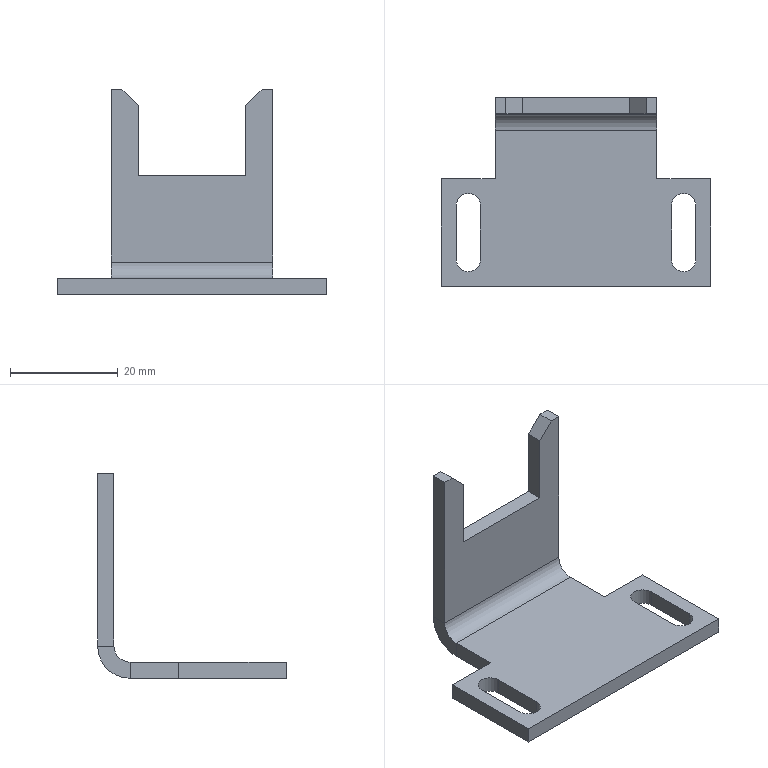Part | NX | features BREP 1 | 1 solid | 32 faces | box 50 x 35 x 38 mm | volume 5974 mm3 | plane 26 | cylinder 6 | commonest cylinder face diameters 4.5 x4 6 x1 12 x1
STEP:
#1=CARTESIAN_POINT('',(-13.,-3.,38.));
#2=VERTEX_POINT('',#1);
#3=CARTESIAN_POINT('',(-15.,-3.,38.));
#4=VERTEX_POINT('',#3);
#5=CARTESIAN_POINT('',(15.,-3.,38.));
#6=DIRECTION('',(-1.,0.,0.));
#7=VECTOR('',#6,1000.);
#8=LINE('',#5,#7);
#9=EDGE_CURVE('',#2,#4,#8,.T.);
#10=ORIENTED_EDGE('',*,*,#9,.F.);
#11=CARTESIAN_POINT('',(-13.,0.,38.));
#12=VERTEX_POINT('',#11);
#13=CARTESIAN_POINT('',(-13.,0.,38.));
#14=DIRECTION('',(0.,1.,0.));
#15=VECTOR('',#14,1000.);
#16=LINE('',#13,#15);
#17=EDGE_CURVE('',#2,#12,#16,.T.);
#18=ORIENTED_EDGE('',*,*,#17,.T.);
#19=CARTESIAN_POINT('',(-15.,0.,38.));
#20=VERTEX_POINT('',#19);
#21=CARTESIAN_POINT('',(15.,0.,38.));
#22=DIRECTION('',(-1.,0.,0.));
#23=VECTOR('',#22,1000.);
#24=LINE('',#21,#23);
#25=EDGE_CURVE('',#12,#20,#24,.T.);
#26=ORIENTED_EDGE('',*,*,#25,.T.);
#27=CARTESIAN_POINT('',(-15.,-3.,38.));
#28=DIRECTION('',(0.,1.,0.));
#29=VECTOR('',#28,1000.);
#30=LINE('',#27,#29);
#31=EDGE_CURVE('',#4,#20,#30,.T.);
#32=ORIENTED_EDGE('',*,*,#31,.F.);
#33=EDGE_LOOP('',(#10,#18,#26,#32));
#34=FACE_BOUND('',#33,.T.);
#35=CARTESIAN_POINT('',(15.,-3.,38.));
#36=DIRECTION('',(0.,0.,1.));
#37=DIRECTION('',(-1.,0.,0.));
#38=AXIS2_PLACEMENT_3D('',#35,#36,#37);
#39=PLANE('',#38);
#40=ADVANCED_FACE('',(#34),#39,.T.);
#41=CARTESIAN_POINT('',(15.,-6.,0.));
#42=VERTEX_POINT('',#41);
#43=CARTESIAN_POINT('',(15.,-6.,3.));
#44=VERTEX_POINT('',#43);
#45=CARTESIAN_POINT('',(15.,-6.,0.));
#46=DIRECTION('',(0.,0.,1.));
#47=VECTOR('',#46,1000.);
#48=LINE('',#45,#47);
#49=EDGE_CURVE('',#42,#44,#48,.T.);
#50=ORIENTED_EDGE('',*,*,#49,.F.);
#51=CARTESIAN_POINT('',(15.,0.,6.));
#52=VERTEX_POINT('',#51);
#53=CARTESIAN_POINT('',(15.,-6.,6.));
#54=DIRECTION('',(-1.,0.,0.));
#55=DIRECTION('',(0.,0.,-1.));
#56=AXIS2_PLACEMENT_3D('',#53,#54,#55);
#57=CIRCLE('',#56,6.);
#58=EDGE_CURVE('',#52,#42,#57,.T.);
#59=ORIENTED_EDGE('',*,*,#58,.F.);
#60=CARTESIAN_POINT('',(15.,-3.,6.));
#61=VERTEX_POINT('',#60);
#62=CARTESIAN_POINT('',(15.,-3.,6.));
#63=DIRECTION('',(0.,1.,0.));
#64=VECTOR('',#63,1000.);
#65=LINE('',#62,#64);
#66=EDGE_CURVE('',#61,#52,#65,.T.);
#67=ORIENTED_EDGE('',*,*,#66,.F.);
#68=CARTESIAN_POINT('',(15.,-6.,6.));
#69=DIRECTION('',(-1.,0.,0.));
#70=DIRECTION('',(0.,0.,-1.));
#71=AXIS2_PLACEMENT_3D('',#68,#69,#70);
#72=CIRCLE('',#71,3.);
#73=EDGE_CURVE('',#61,#44,#72,.T.);
#74=ORIENTED_EDGE('',*,*,#73,.T.);
#75=EDGE_LOOP('',(#50,#59,#67,#74));
#76=FACE_BOUND('',#75,.T.);
#77=CARTESIAN_POINT('',(15.,-6.,0.));
#78=DIRECTION('',(1.,0.,0.));
#79=DIRECTION('',(0.,0.,1.));
#80=AXIS2_PLACEMENT_3D('',#77,#78,#79);
#81=PLANE('',#80);
#82=ADVANCED_FACE('',(#76),#81,.T.);
#83=CARTESIAN_POINT('',(15.,-15.,0.));
#84=VERTEX_POINT('',#83);
#85=CARTESIAN_POINT('',(15.,-15.,3.));
#86=VERTEX_POINT('',#85);
#87=CARTESIAN_POINT('',(15.,-15.,6.));
#88=DIRECTION('',(0.,0.,1.));
#89=VECTOR('',#88,1000.);
#90=LINE('',#87,#89);
#91=EDGE_CURVE('',#84,#86,#90,.T.);
#92=ORIENTED_EDGE('',*,*,#91,.F.);
#93=CARTESIAN_POINT('',(15.,0.,0.));
#94=DIRECTION('',(0.,-1.,0.));
#95=VECTOR('',#94,1000.);
#96=LINE('',#93,#95);
#97=EDGE_CURVE('',#42,#84,#96,.T.);
#98=ORIENTED_EDGE('',*,*,#97,.F.);
#99=ORIENTED_EDGE('',*,*,#49,.T.);
#100=CARTESIAN_POINT('',(15.,0.,3.));
#101=DIRECTION('',(0.,-1.,0.));
#102=VECTOR('',#101,1000.);
#103=LINE('',#100,#102);
#104=EDGE_CURVE('',#44,#86,#103,.T.);
#105=ORIENTED_EDGE('',*,*,#104,.T.);
#106=EDGE_LOOP('',(#92,#98,#99,#105));
#107=FACE_BOUND('',#106,.T.);
#108=CARTESIAN_POINT('',(15.,-3.,6.));
#109=DIRECTION('',(1.,0.,0.));
#110=DIRECTION('',(0.,0.,1.));
#111=AXIS2_PLACEMENT_3D('',#108,#109,#110);
#112=PLANE('',#111);
#113=ADVANCED_FACE('',(#107),#112,.T.);
#114=CARTESIAN_POINT('',(-15.,0.,6.));
#115=VERTEX_POINT('',#114);
#116=CARTESIAN_POINT('',(-15.,-3.,6.));
#117=VERTEX_POINT('',#116);
#118=CARTESIAN_POINT('',(-15.,0.,6.));
#119=DIRECTION('',(0.,-1.,0.));
#120=VECTOR('',#119,1000.);
#121=LINE('',#118,#120);
#122=EDGE_CURVE('',#115,#117,#121,.T.);
#123=ORIENTED_EDGE('',*,*,#122,.F.);
#124=CARTESIAN_POINT('',(-15.,-6.,0.));
#125=VERTEX_POINT('',#124);
#126=CARTESIAN_POINT('',(-15.,-6.,6.));
#127=DIRECTION('',(-1.,0.,0.));
#128=DIRECTION('',(0.,0.,-1.));
#129=AXIS2_PLACEMENT_3D('',#126,#127,#128);
#130=CIRCLE('',#129,6.);
#131=EDGE_CURVE('',#115,#125,#130,.T.);
#132=ORIENTED_EDGE('',*,*,#131,.T.);
#133=CARTESIAN_POINT('',(-15.,-6.,3.));
#134=VERTEX_POINT('',#133);
#135=CARTESIAN_POINT('',(-15.,-6.,3.));
#136=DIRECTION('',(0.,0.,-1.));
#137=VECTOR('',#136,1000.);
#138=LINE('',#135,#137);
#139=EDGE_CURVE('',#134,#125,#138,.T.);
#140=ORIENTED_EDGE('',*,*,#139,.F.);
#141=CARTESIAN_POINT('',(-15.,-6.,6.));
#142=DIRECTION('',(-1.,0.,0.));
#143=DIRECTION('',(0.,0.,-1.));
#144=AXIS2_PLACEMENT_3D('',#141,#142,#143);
#145=CIRCLE('',#144,3.);
#146=EDGE_CURVE('',#117,#134,#145,.T.);
#147=ORIENTED_EDGE('',*,*,#146,.F.);
#148=EDGE_LOOP('',(#123,#132,#140,#147));
#149=FACE_BOUND('',#148,.T.);
#150=CARTESIAN_POINT('',(-15.,0.,6.));
#151=DIRECTION('',(-1.,0.,0.));
#152=DIRECTION('',(0.,0.,-1.));
#153=AXIS2_PLACEMENT_3D('',#150,#151,#152);
#154=PLANE('',#153);
#155=ADVANCED_FACE('',(#149),#154,.T.);
#156=CARTESIAN_POINT('',(-15.,0.,38.));
#157=DIRECTION('',(0.,0.,-1.));
#158=VECTOR('',#157,1000.);
#159=LINE('',#156,#158);
#160=EDGE_CURVE('',#20,#115,#159,.T.);
#161=ORIENTED_EDGE('',*,*,#160,.T.);
#162=ORIENTED_EDGE('',*,*,#122,.T.);
#163=CARTESIAN_POINT('',(-15.,-3.,38.));
#164=DIRECTION('',(0.,0.,-1.));
#165=VECTOR('',#164,1000.);
#166=LINE('',#163,#165);
#167=EDGE_CURVE('',#4,#117,#166,.T.);
#168=ORIENTED_EDGE('',*,*,#167,.F.);
#169=ORIENTED_EDGE('',*,*,#31,.T.);
#170=EDGE_LOOP('',(#161,#162,#168,#169));
#171=FACE_BOUND('',#170,.T.);
#172=CARTESIAN_POINT('',(-15.,-6.,3.));
#173=DIRECTION('',(-1.,0.,0.));
#174=DIRECTION('',(0.,0.,-1.));
#175=AXIS2_PLACEMENT_3D('',#172,#173,#174);
#176=PLANE('',#175);
#177=ADVANCED_FACE('',(#171),#176,.T.);
#178=CARTESIAN_POINT('',(17.75,-30.,3.));
#179=VERTEX_POINT('',#178);
#180=CARTESIAN_POINT('',(22.25,-30.,3.));
#181=VERTEX_POINT('',#180);
#182=CARTESIAN_POINT('',(20.,-30.,3.));
#183=DIRECTION('',(0.,0.,1.));
#184=DIRECTION('',(1.,0.,0.));
#185=AXIS2_PLACEMENT_3D('',#182,#183,#184);
#186=CIRCLE('',#185,2.25);
#187=EDGE_CURVE('',#179,#181,#186,.T.);
#188=ORIENTED_EDGE('',*,*,#187,.F.);
#189=CARTESIAN_POINT('',(17.75,-20.,3.));
#190=VERTEX_POINT('',#189);
#191=CARTESIAN_POINT('',(17.75,-20.,3.));
#192=DIRECTION('',(0.,-1.,0.));
#193=VECTOR('',#192,1000.);
#194=LINE('',#191,#193);
#195=EDGE_CURVE('',#190,#179,#194,.T.);
#196=ORIENTED_EDGE('',*,*,#195,.F.);
#197=CARTESIAN_POINT('',(22.25,-20.,3.));
#198=VERTEX_POINT('',#197);
#199=CARTESIAN_POINT('',(20.,-20.,3.));
#200=DIRECTION('',(0.,0.,1.));
#201=DIRECTION('',(1.,0.,0.));
#202=AXIS2_PLACEMENT_3D('',#199,#200,#201);
#203=CIRCLE('',#202,2.25);
#204=EDGE_CURVE('',#198,#190,#203,.T.);
#205=ORIENTED_EDGE('',*,*,#204,.F.);
#206=CARTESIAN_POINT('',(22.25,-20.,3.));
#207=DIRECTION('',(0.,1.,0.));
#208=VECTOR('',#207,1000.);
#209=LINE('',#206,#208);
#210=EDGE_CURVE('',#181,#198,#209,.T.);
#211=ORIENTED_EDGE('',*,*,#210,.F.);
#212=EDGE_LOOP('',(#188,#196,#205,#211));
#213=FACE_BOUND('',#212,.T.);
#214=CARTESIAN_POINT('',(-22.25,-30.,3.));
#215=VERTEX_POINT('',#214);
#216=CARTESIAN_POINT('',(-17.75,-30.,3.));
#217=VERTEX_POINT('',#216);
#218=CARTESIAN_POINT('',(-20.,-30.,3.));
#219=DIRECTION('',(0.,0.,1.));
#220=DIRECTION('',(1.,0.,0.));
#221=AXIS2_PLACEMENT_3D('',#218,#219,#220);
#222=CIRCLE('',#221,2.25);
#223=EDGE_CURVE('',#215,#217,#222,.T.);
#224=ORIENTED_EDGE('',*,*,#223,.F.);
#225=CARTESIAN_POINT('',(-22.25,-20.,3.));
#226=VERTEX_POINT('',#225);
#227=CARTESIAN_POINT('',(-22.25,-20.,3.));
#228=DIRECTION('',(0.,-1.,0.));
#229=VECTOR('',#228,1000.);
#230=LINE('',#227,#229);
#231=EDGE_CURVE('',#226,#215,#230,.T.);
#232=ORIENTED_EDGE('',*,*,#231,.F.);
#233=CARTESIAN_POINT('',(-17.75,-20.,3.));
#234=VERTEX_POINT('',#233);
#235=CARTESIAN_POINT('',(-20.,-20.,3.));
#236=DIRECTION('',(0.,0.,1.));
#237=DIRECTION('',(1.,0.,0.));
#238=AXIS2_PLACEMENT_3D('',#235,#236,#237);
#239=CIRCLE('',#238,2.25);
#240=EDGE_CURVE('',#234,#226,#239,.T.);
#241=ORIENTED_EDGE('',*,*,#240,.F.);
#242=CARTESIAN_POINT('',(-17.75,-20.,3.));
#243=DIRECTION('',(0.,1.,0.));
#244=VECTOR('',#243,1000.);
#245=LINE('',#242,#244);
#246=EDGE_CURVE('',#217,#234,#245,.T.);
#247=ORIENTED_EDGE('',*,*,#246,.F.);
#248=EDGE_LOOP('',(#224,#232,#241,#247));
#249=FACE_BOUND('',#248,.T.);
#250=CARTESIAN_POINT('',(-15.,-15.,3.));
#251=VERTEX_POINT('',#250);
#252=CARTESIAN_POINT('',(-15.,0.,3.));
#253=DIRECTION('',(0.,-1.,0.));
#254=VECTOR('',#253,1000.);
#255=LINE('',#252,#254);
#256=EDGE_CURVE('',#134,#251,#255,.T.);
#257=ORIENTED_EDGE('',*,*,#256,.T.);
#258=CARTESIAN_POINT('',(-25.,-15.,3.));
#259=VERTEX_POINT('',#258);
#260=CARTESIAN_POINT('',(25.,-15.,3.));
#261=DIRECTION('',(-1.,0.,0.));
#262=VECTOR('',#261,1000.);
#263=LINE('',#260,#262);
#264=EDGE_CURVE('',#251,#259,#263,.T.);
#265=ORIENTED_EDGE('',*,*,#264,.T.);
#266=CARTESIAN_POINT('',(-25.,-35.,3.));
#267=VERTEX_POINT('',#266);
#268=CARTESIAN_POINT('',(-25.,-15.,3.));
#269=DIRECTION('',(0.,-1.,0.));
#270=VECTOR('',#269,1000.);
#271=LINE('',#268,#270);
#272=EDGE_CURVE('',#259,#267,#271,.T.);
#273=ORIENTED_EDGE('',*,*,#272,.T.);
#274=CARTESIAN_POINT('',(25.,-35.,3.));
#275=VERTEX_POINT('',#274);
#276=CARTESIAN_POINT('',(15.,-35.,3.));
#277=DIRECTION('',(-1.,0.,0.));
#278=VECTOR('',#277,1000.);
#279=LINE('',#276,#278);
#280=EDGE_CURVE('',#275,#267,#279,.T.);
#281=ORIENTED_EDGE('',*,*,#280,.F.);
#282=CARTESIAN_POINT('',(25.,-15.,3.));
#283=VERTEX_POINT('',#282);
#284=CARTESIAN_POINT('',(25.,-15.,3.));
#285=DIRECTION('',(0.,1.,0.));
#286=VECTOR('',#285,1000.);
#287=LINE('',#284,#286);
#288=EDGE_CURVE('',#275,#283,#287,.T.);
#289=ORIENTED_EDGE('',*,*,#288,.T.);
#290=CARTESIAN_POINT('',(25.,-15.,3.));
#291=DIRECTION('',(-1.,0.,0.));
#292=VECTOR('',#291,1000.);
#293=LINE('',#290,#292);
#294=EDGE_CURVE('',#283,#86,#293,.T.);
#295=ORIENTED_EDGE('',*,*,#294,.T.);
#296=ORIENTED_EDGE('',*,*,#104,.F.);
#297=CARTESIAN_POINT('',(15.,-6.,3.));
#298=DIRECTION('',(-1.,0.,0.));
#299=VECTOR('',#298,1000.);
#300=LINE('',#297,#299);
#301=EDGE_CURVE('',#44,#134,#300,.T.);
#302=ORIENTED_EDGE('',*,*,#301,.T.);
#303=EDGE_LOOP('',(#257,#265,#273,#281,#289,#295,#296,#302));
#304=FACE_BOUND('',#303,.T.);
#305=CARTESIAN_POINT('',(15.,0.,3.));
#306=DIRECTION('',(0.,0.,-1.));
#307=DIRECTION('',(0.,-1.,0.));
#308=AXIS2_PLACEMENT_3D('',#305,#306,#307);
#309=PLANE('',#308);
#310=ADVANCED_FACE('',(#213,#249,#304),#309,.F.);
#311=ORIENTED_EDGE('',*,*,#280,.T.);
#312=CARTESIAN_POINT('',(-25.,-35.,0.));
#313=VERTEX_POINT('',#312);
#314=CARTESIAN_POINT('',(-25.,-35.,-53.852));
#315=DIRECTION('',(0.,0.,1.));
#316=VECTOR('',#315,1000.);
#317=LINE('',#314,#316);
#318=EDGE_CURVE('',#313,#267,#317,.T.);
#319=ORIENTED_EDGE('',*,*,#318,.F.);
#320=CARTESIAN_POINT('',(25.,-35.,0.));
#321=VERTEX_POINT('',#320);
#322=CARTESIAN_POINT('',(15.,-35.,0.));
#323=DIRECTION('',(-1.,0.,0.));
#324=VECTOR('',#323,1000.);
#325=LINE('',#322,#324);
#326=EDGE_CURVE('',#321,#313,#325,.T.);
#327=ORIENTED_EDGE('',*,*,#326,.F.);
#328=CARTESIAN_POINT('',(25.,-35.,-53.852));
#329=DIRECTION('',(0.,0.,1.));
#330=VECTOR('',#329,1000.);
#331=LINE('',#328,#330);
#332=EDGE_CURVE('',#321,#275,#331,.T.);
#333=ORIENTED_EDGE('',*,*,#332,.T.);
#334=EDGE_LOOP('',(#311,#319,#327,#333));
#335=FACE_BOUND('',#334,.T.);
#336=CARTESIAN_POINT('',(15.,-35.,0.));
#337=DIRECTION('',(0.,-1.,0.));
#338=DIRECTION('',(0.,0.,1.));
#339=AXIS2_PLACEMENT_3D('',#336,#337,#338);
#340=PLANE('',#339);
#341=ADVANCED_FACE('',(#335),#340,.T.);
#342=CARTESIAN_POINT('',(17.75,-20.,0.));
#343=VERTEX_POINT('',#342);
#344=CARTESIAN_POINT('',(17.75,-30.,0.));
#345=VERTEX_POINT('',#344);
#346=CARTESIAN_POINT('',(17.75,-20.,0.));
#347=DIRECTION('',(0.,-1.,0.));
#348=VECTOR('',#347,1000.);
#349=LINE('',#346,#348);
#350=EDGE_CURVE('',#343,#345,#349,.T.);
#351=ORIENTED_EDGE('',*,*,#350,.T.);
#352=CARTESIAN_POINT('',(22.25,-30.,0.));
#353=VERTEX_POINT('',#352);
#354=CARTESIAN_POINT('',(20.,-30.,0.));
#355=DIRECTION('',(0.,0.,1.));
#356=DIRECTION('',(0.,1.,0.));
#357=AXIS2_PLACEMENT_3D('',#354,#355,#356);
#358=CIRCLE('',#357,2.25);
#359=EDGE_CURVE('',#345,#353,#358,.T.);
#360=ORIENTED_EDGE('',*,*,#359,.T.);
#361=CARTESIAN_POINT('',(22.25,-20.,0.));
#362=VERTEX_POINT('',#361);
#363=CARTESIAN_POINT('',(22.25,-20.,0.));
#364=DIRECTION('',(0.,1.,0.));
#365=VECTOR('',#364,1000.);
#366=LINE('',#363,#365);
#367=EDGE_CURVE('',#353,#362,#366,.T.);
#368=ORIENTED_EDGE('',*,*,#367,.T.);
#369=CARTESIAN_POINT('',(20.,-20.,0.));
#370=DIRECTION('',(0.,0.,1.));
#371=DIRECTION('',(0.,1.,0.));
#372=AXIS2_PLACEMENT_3D('',#369,#370,#371);
#373=CIRCLE('',#372,2.25);
#374=EDGE_CURVE('',#362,#343,#373,.T.);
#375=ORIENTED_EDGE('',*,*,#374,.T.);
#376=EDGE_LOOP('',(#351,#360,#368,#375));
#377=FACE_BOUND('',#376,.T.);
#378=CARTESIAN_POINT('',(-22.25,-20.,0.));
#379=VERTEX_POINT('',#378);
#380=CARTESIAN_POINT('',(-22.25,-30.,0.));
#381=VERTEX_POINT('',#380);
#382=CARTESIAN_POINT('',(-22.25,-20.,0.));
#383=DIRECTION('',(0.,-1.,0.));
#384=VECTOR('',#383,1000.);
#385=LINE('',#382,#384);
#386=EDGE_CURVE('',#379,#381,#385,.T.);
#387=ORIENTED_EDGE('',*,*,#386,.T.);
#388=CARTESIAN_POINT('',(-17.75,-30.,0.));
#389=VERTEX_POINT('',#388);
#390=CARTESIAN_POINT('',(-20.,-30.,0.));
#391=DIRECTION('',(0.,0.,1.));
#392=DIRECTION('',(0.,1.,0.));
#393=AXIS2_PLACEMENT_3D('',#390,#391,#392);
#394=CIRCLE('',#393,2.25);
#395=EDGE_CURVE('',#381,#389,#394,.T.);
#396=ORIENTED_EDGE('',*,*,#395,.T.);
#397=CARTESIAN_POINT('',(-17.75,-20.,0.));
#398=VERTEX_POINT('',#397);
#399=CARTESIAN_POINT('',(-17.75,-20.,0.));
#400=DIRECTION('',(0.,1.,0.));
#401=VECTOR('',#400,1000.);
#402=LINE('',#399,#401);
#403=EDGE_CURVE('',#389,#398,#402,.T.);
#404=ORIENTED_EDGE('',*,*,#403,.T.);
#405=CARTESIAN_POINT('',(-20.,-20.,0.));
#406=DIRECTION('',(0.,0.,1.));
#407=DIRECTION('',(0.,1.,0.));
#408=AXIS2_PLACEMENT_3D('',#405,#406,#407);
#409=CIRCLE('',#408,2.25);
#410=EDGE_CURVE('',#398,#379,#409,.T.);
#411=ORIENTED_EDGE('',*,*,#410,.T.);
#412=EDGE_LOOP('',(#387,#396,#404,#411));
#413=FACE_BOUND('',#412,.T.);
#414=ORIENTED_EDGE('',*,*,#97,.T.);
#415=CARTESIAN_POINT('',(25.,-15.,0.));
#416=VERTEX_POINT('',#415);
#417=CARTESIAN_POINT('',(25.,-15.,0.));
#418=DIRECTION('',(-1.,0.,0.));
#419=VECTOR('',#418,1000.);
#420=LINE('',#417,#419);
#421=EDGE_CURVE('',#416,#84,#420,.T.);
#422=ORIENTED_EDGE('',*,*,#421,.F.);
#423=CARTESIAN_POINT('',(25.,-15.,0.));
#424=DIRECTION('',(0.,1.,0.));
#425=VECTOR('',#424,1000.);
#426=LINE('',#423,#425);
#427=EDGE_CURVE('',#321,#416,#426,.T.);
#428=ORIENTED_EDGE('',*,*,#427,.F.);
#429=ORIENTED_EDGE('',*,*,#326,.T.);
#430=CARTESIAN_POINT('',(-25.,-15.,0.));
#431=VERTEX_POINT('',#430);
#432=CARTESIAN_POINT('',(-25.,-15.,0.));
#433=DIRECTION('',(0.,-1.,0.));
#434=VECTOR('',#433,1000.);
#435=LINE('',#432,#434);
#436=EDGE_CURVE('',#431,#313,#435,.T.);
#437=ORIENTED_EDGE('',*,*,#436,.F.);
#438=CARTESIAN_POINT('',(-15.,-15.,0.));
#439=VERTEX_POINT('',#438);
#440=CARTESIAN_POINT('',(25.,-15.,0.));
#441=DIRECTION('',(-1.,0.,0.));
#442=VECTOR('',#441,1000.);
#443=LINE('',#440,#442);
#444=EDGE_CURVE('',#439,#431,#443,.T.);
#445=ORIENTED_EDGE('',*,*,#444,.F.);
#446=CARTESIAN_POINT('',(-15.,0.,0.));
#447=DIRECTION('',(0.,-1.,0.));
#448=VECTOR('',#447,1000.);
#449=LINE('',#446,#448);
#450=EDGE_CURVE('',#125,#439,#449,.T.);
#451=ORIENTED_EDGE('',*,*,#450,.F.);
#452=CARTESIAN_POINT('',(15.,-6.,0.));
#453=DIRECTION('',(-1.,0.,0.));
#454=VECTOR('',#453,1000.);
#455=LINE('',#452,#454);
#456=EDGE_CURVE('',#42,#125,#455,.T.);
#457=ORIENTED_EDGE('',*,*,#456,.F.);
#458=EDGE_LOOP('',(#414,#422,#428,#429,#437,#445,#451,#457));
#459=FACE_BOUND('',#458,.T.);
#460=CARTESIAN_POINT('',(15.,0.,0.));
#461=DIRECTION('',(0.,0.,-1.));
#462=DIRECTION('',(0.,-1.,0.));
#463=AXIS2_PLACEMENT_3D('',#460,#461,#462);
#464=PLANE('',#463);
#465=ADVANCED_FACE('',(#377,#413,#459),#464,.T.);
#466=ORIENTED_EDGE('',*,*,#131,.F.);
#467=CARTESIAN_POINT('',(15.,0.,6.));
#468=DIRECTION('',(-1.,0.,0.));
#469=VECTOR('',#468,1000.);
#470=LINE('',#467,#469);
#471=EDGE_CURVE('',#52,#115,#470,.T.);
#472=ORIENTED_EDGE('',*,*,#471,.F.);
#473=ORIENTED_EDGE('',*,*,#58,.T.);
#474=ORIENTED_EDGE('',*,*,#456,.T.);
#475=EDGE_LOOP('',(#466,#472,#473,#474));
#476=FACE_BOUND('',#475,.T.);
#477=CARTESIAN_POINT('',(15.,-6.,6.));
#478=DIRECTION('',(-1.,0.,0.));
#479=DIRECTION('',(0.,0.,-1.));
#480=AXIS2_PLACEMENT_3D('',#477,#478,#479);
#481=CYLINDRICAL_SURFACE('',#480,6.);
#482=ADVANCED_FACE('',(#476),#481,.T.);
#483=ORIENTED_EDGE('',*,*,#25,.F.);
#484=CARTESIAN_POINT('',(-10.,0.,35.));
#485=VERTEX_POINT('',#484);
#486=CARTESIAN_POINT('',(1.,0.,24.));
#487=DIRECTION('',(0.7071,0.,-0.7071));
#488=VECTOR('',#487,1000.);
#489=LINE('',#486,#488);
#490=EDGE_CURVE('',#12,#485,#489,.T.);
#491=ORIENTED_EDGE('',*,*,#490,.T.);
#492=CARTESIAN_POINT('',(-10.,0.,22.));
#493=VERTEX_POINT('',#492);
#494=CARTESIAN_POINT('',(-10.,0.,38.));
#495=DIRECTION('',(0.,0.,-1.));
#496=VECTOR('',#495,1000.);
#497=LINE('',#494,#496);
#498=EDGE_CURVE('',#485,#493,#497,.T.);
#499=ORIENTED_EDGE('',*,*,#498,.T.);
#500=CARTESIAN_POINT('',(10.,0.,22.));
#501=VERTEX_POINT('',#500);
#502=CARTESIAN_POINT('',(10.,0.,22.));
#503=DIRECTION('',(1.,0.,0.));
#504=VECTOR('',#503,1000.);
#505=LINE('',#502,#504);
#506=EDGE_CURVE('',#493,#501,#505,.T.);
#507=ORIENTED_EDGE('',*,*,#506,.T.);
#508=CARTESIAN_POINT('',(10.,0.,35.));
#509=VERTEX_POINT('',#508);
#510=CARTESIAN_POINT('',(10.,0.,38.));
#511=DIRECTION('',(0.,0.,1.));
#512=VECTOR('',#511,1000.);
#513=LINE('',#510,#512);
#514=EDGE_CURVE('',#501,#509,#513,.T.);
#515=ORIENTED_EDGE('',*,*,#514,.T.);
#516=CARTESIAN_POINT('',(13.,0.,38.));
#517=VERTEX_POINT('',#516);
#518=CARTESIAN_POINT('',(14.,0.,39.));
#519=DIRECTION('',(0.7071,0.,0.7071));
#520=VECTOR('',#519,1000.);
#521=LINE('',#518,#520);
#522=EDGE_CURVE('',#509,#517,#521,.T.);
#523=ORIENTED_EDGE('',*,*,#522,.T.);
#524=CARTESIAN_POINT('',(15.,0.,38.));
#525=VERTEX_POINT('',#524);
#526=CARTESIAN_POINT('',(15.,0.,38.));
#527=DIRECTION('',(-1.,0.,0.));
#528=VECTOR('',#527,1000.);
#529=LINE('',#526,#528);
#530=EDGE_CURVE('',#525,#517,#529,.T.);
#531=ORIENTED_EDGE('',*,*,#530,.F.);
#532=CARTESIAN_POINT('',(15.,0.,38.));
#533=DIRECTION('',(0.,0.,-1.));
#534=VECTOR('',#533,1000.);
#535=LINE('',#532,#534);
#536=EDGE_CURVE('',#525,#52,#535,.T.);
#537=ORIENTED_EDGE('',*,*,#536,.T.);
#538=ORIENTED_EDGE('',*,*,#471,.T.);
#539=ORIENTED_EDGE('',*,*,#160,.F.);
#540=EDGE_LOOP('',(#483,#491,#499,#507,#515,#523,#531,#537,#538,#539));
#541=FACE_BOUND('',#540,.T.);
#542=CARTESIAN_POINT('',(15.,0.,38.));
#543=DIRECTION('',(0.,1.,0.));
#544=DIRECTION('',(0.,0.,-1.));
#545=AXIS2_PLACEMENT_3D('',#542,#543,#544);
#546=PLANE('',#545);
#547=ADVANCED_FACE('',(#541),#546,.T.);
#548=ORIENTED_EDGE('',*,*,#530,.T.);
#549=CARTESIAN_POINT('',(13.,-3.,38.));
#550=VERTEX_POINT('',#549);
#551=CARTESIAN_POINT('',(13.,-3.,38.));
#552=DIRECTION('',(0.,-1.,0.));
#553=VECTOR('',#552,1000.);
#554=LINE('',#551,#553);
#555=EDGE_CURVE('',#517,#550,#554,.T.);
#556=ORIENTED_EDGE('',*,*,#555,.T.);
#557=CARTESIAN_POINT('',(15.,-3.,38.));
#558=VERTEX_POINT('',#557);
#559=CARTESIAN_POINT('',(15.,-3.,38.));
#560=DIRECTION('',(-1.,0.,0.));
#561=VECTOR('',#560,1000.);
#562=LINE('',#559,#561);
#563=EDGE_CURVE('',#558,#550,#562,.T.);
#564=ORIENTED_EDGE('',*,*,#563,.F.);
#565=CARTESIAN_POINT('',(15.,-3.,38.));
#566=DIRECTION('',(0.,1.,0.));
#567=VECTOR('',#566,1000.);
#568=LINE('',#565,#567);
#569=EDGE_CURVE('',#558,#525,#568,.T.);
#570=ORIENTED_EDGE('',*,*,#569,.T.);
#571=EDGE_LOOP('',(#548,#556,#564,#570));
#572=FACE_BOUND('',#571,.T.);
#573=CARTESIAN_POINT('',(15.,-3.,38.));
#574=DIRECTION('',(0.,0.,1.));
#575=DIRECTION('',(-1.,0.,0.));
#576=AXIS2_PLACEMENT_3D('',#573,#574,#575);
#577=PLANE('',#576);
#578=ADVANCED_FACE('',(#572),#577,.T.);
#579=CARTESIAN_POINT('',(-10.,-3.,35.));
#580=VERTEX_POINT('',#579);
#581=CARTESIAN_POINT('',(-10.,-3.,22.));
#582=VERTEX_POINT('',#581);
#583=CARTESIAN_POINT('',(-10.,-3.,38.));
#584=DIRECTION('',(0.,0.,-1.));
#585=VECTOR('',#584,1000.);
#586=LINE('',#583,#585);
#587=EDGE_CURVE('',#580,#582,#586,.T.);
#588=ORIENTED_EDGE('',*,*,#587,.F.);
#589=CARTESIAN_POINT('',(-10.,-3.,35.));
#590=DIRECTION('',(-0.7071,0.,0.7071));
#591=VECTOR('',#590,1000.);
#592=LINE('',#589,#591);
#593=EDGE_CURVE('',#580,#2,#592,.T.);
#594=ORIENTED_EDGE('',*,*,#593,.T.);
#595=ORIENTED_EDGE('',*,*,#9,.T.);
#596=ORIENTED_EDGE('',*,*,#167,.T.);
#597=CARTESIAN_POINT('',(15.,-3.,6.));
#598=DIRECTION('',(-1.,0.,0.));
#599=VECTOR('',#598,1000.);
#600=LINE('',#597,#599);
#601=EDGE_CURVE('',#61,#117,#600,.T.);
#602=ORIENTED_EDGE('',*,*,#601,.F.);
#603=CARTESIAN_POINT('',(15.,-3.,38.));
#604=DIRECTION('',(0.,0.,-1.));
#605=VECTOR('',#604,1000.);
#606=LINE('',#603,#605);
#607=EDGE_CURVE('',#558,#61,#606,.T.);
#608=ORIENTED_EDGE('',*,*,#607,.F.);
#609=ORIENTED_EDGE('',*,*,#563,.T.);
#610=CARTESIAN_POINT('',(10.,-3.,35.));
#611=VERTEX_POINT('',#610);
#612=CARTESIAN_POINT('',(13.,-3.,38.));
#613=DIRECTION('',(-0.7071,0.,-0.7071));
#614=VECTOR('',#613,1000.);
#615=LINE('',#612,#614);
#616=EDGE_CURVE('',#550,#611,#615,.T.);
#617=ORIENTED_EDGE('',*,*,#616,.T.);
#618=CARTESIAN_POINT('',(10.,-3.,22.));
#619=VERTEX_POINT('',#618);
#620=CARTESIAN_POINT('',(10.,-3.,38.));
#621=DIRECTION('',(0.,0.,1.));
#622=VECTOR('',#621,1000.);
#623=LINE('',#620,#622);
#624=EDGE_CURVE('',#619,#611,#623,.T.);
#625=ORIENTED_EDGE('',*,*,#624,.F.);
#626=CARTESIAN_POINT('',(10.,-3.,22.));
#627=DIRECTION('',(1.,0.,0.));
#628=VECTOR('',#627,1000.);
#629=LINE('',#626,#628);
#630=EDGE_CURVE('',#582,#619,#629,.T.);
#631=ORIENTED_EDGE('',*,*,#630,.F.);
#632=EDGE_LOOP('',(#588,#594,#595,#596,#602,#608,#609,#617,#625,#631));
#633=FACE_BOUND('',#632,.T.);
#634=CARTESIAN_POINT('',(15.,-3.,38.));
#635=DIRECTION('',(0.,1.,0.));
#636=DIRECTION('',(0.,0.,-1.));
#637=AXIS2_PLACEMENT_3D('',#634,#635,#636);
#638=PLANE('',#637);
#639=ADVANCED_FACE('',(#633),#638,.F.);
#640=ORIENTED_EDGE('',*,*,#146,.T.);
#641=ORIENTED_EDGE('',*,*,#301,.F.);
#642=ORIENTED_EDGE('',*,*,#73,.F.);
#643=ORIENTED_EDGE('',*,*,#601,.T.);
#644=EDGE_LOOP('',(#640,#641,#642,#643));
#645=FACE_BOUND('',#644,.T.);
#646=CARTESIAN_POINT('',(15.,-6.,6.));
#647=DIRECTION('',(-1.,0.,0.));
#648=DIRECTION('',(0.,0.,-1.));
#649=AXIS2_PLACEMENT_3D('',#646,#647,#648);
#650=CYLINDRICAL_SURFACE('',#649,3.);
#651=ADVANCED_FACE('',(#645),#650,.F.);
#652=ORIENTED_EDGE('',*,*,#607,.T.);
#653=ORIENTED_EDGE('',*,*,#66,.T.);
#654=ORIENTED_EDGE('',*,*,#536,.F.);
#655=ORIENTED_EDGE('',*,*,#569,.F.);
#656=EDGE_LOOP('',(#652,#653,#654,#655));
#657=FACE_BOUND('',#656,.T.);
#658=CARTESIAN_POINT('',(15.,-6.,6.));
#659=DIRECTION('',(1.,0.,0.));
#660=DIRECTION('',(0.,0.,1.));
#661=AXIS2_PLACEMENT_3D('',#658,#659,#660);
#662=PLANE('',#661);
#663=ADVANCED_FACE('',(#657),#662,.T.);
#664=ORIENTED_EDGE('',*,*,#450,.T.);
#665=CARTESIAN_POINT('',(-15.,-15.,6.));
#666=DIRECTION('',(0.,0.,1.));
#667=VECTOR('',#666,1000.);
#668=LINE('',#665,#667);
#669=EDGE_CURVE('',#439,#251,#668,.T.);
#670=ORIENTED_EDGE('',*,*,#669,.T.);
#671=ORIENTED_EDGE('',*,*,#256,.F.);
#672=ORIENTED_EDGE('',*,*,#139,.T.);
#673=EDGE_LOOP('',(#664,#670,#671,#672));
#674=FACE_BOUND('',#673,.T.);
#675=CARTESIAN_POINT('',(-15.,-6.,6.));
#676=DIRECTION('',(1.,0.,0.));
#677=DIRECTION('',(0.,0.,1.));
#678=AXIS2_PLACEMENT_3D('',#675,#676,#677);
#679=PLANE('',#678);
#680=ADVANCED_FACE('',(#674),#679,.F.);
#681=ORIENTED_EDGE('',*,*,#498,.F.);
#682=CARTESIAN_POINT('',(-10.,-3.,35.));
#683=DIRECTION('',(0.,-1.,0.));
#684=VECTOR('',#683,1000.);
#685=LINE('',#682,#684);
#686=EDGE_CURVE('',#485,#580,#685,.T.);
#687=ORIENTED_EDGE('',*,*,#686,.T.);
#688=ORIENTED_EDGE('',*,*,#587,.T.);
#689=CARTESIAN_POINT('',(-10.,25.612,22.));
#690=DIRECTION('',(0.,-1.,0.));
#691=VECTOR('',#690,1000.);
#692=LINE('',#689,#691);
#693=EDGE_CURVE('',#493,#582,#692,.T.);
#694=ORIENTED_EDGE('',*,*,#693,.F.);
#695=EDGE_LOOP('',(#681,#687,#688,#694));
#696=FACE_BOUND('',#695,.T.);
#697=CARTESIAN_POINT('',(-10.,25.612,38.));
#698=DIRECTION('',(-1.,0.,0.));
#699=DIRECTION('',(0.,0.,-1.));
#700=AXIS2_PLACEMENT_3D('',#697,#698,#699);
#701=PLANE('',#700);
#702=ADVANCED_FACE('',(#696),#701,.F.);
#703=ORIENTED_EDGE('',*,*,#693,.T.);
#704=ORIENTED_EDGE('',*,*,#630,.T.);
#705=CARTESIAN_POINT('',(10.,25.612,22.));
#706=DIRECTION('',(0.,-1.,0.));
#707=VECTOR('',#706,1000.);
#708=LINE('',#705,#707);
#709=EDGE_CURVE('',#501,#619,#708,.T.);
#710=ORIENTED_EDGE('',*,*,#709,.F.);
#711=ORIENTED_EDGE('',*,*,#506,.F.);
#712=EDGE_LOOP('',(#703,#704,#710,#711));
#713=FACE_BOUND('',#712,.T.);
#714=CARTESIAN_POINT('',(10.,25.612,22.));
#715=DIRECTION('',(0.,0.,-1.));
#716=DIRECTION('',(1.,0.,0.));
#717=AXIS2_PLACEMENT_3D('',#714,#715,#716);
#718=PLANE('',#717);
#719=ADVANCED_FACE('',(#713),#718,.F.);
#720=ORIENTED_EDGE('',*,*,#624,.T.);
#721=CARTESIAN_POINT('',(10.,0.,35.));
#722=DIRECTION('',(0.,1.,0.));
#723=VECTOR('',#722,1000.);
#724=LINE('',#721,#723);
#725=EDGE_CURVE('',#611,#509,#724,.T.);
#726=ORIENTED_EDGE('',*,*,#725,.T.);
#727=ORIENTED_EDGE('',*,*,#514,.F.);
#728=ORIENTED_EDGE('',*,*,#709,.T.);
#729=EDGE_LOOP('',(#720,#726,#727,#728));
#730=FACE_BOUND('',#729,.T.);
#731=CARTESIAN_POINT('',(10.,25.612,38.));
#732=DIRECTION('',(1.,0.,0.));
#733=DIRECTION('',(0.,0.,1.));
#734=AXIS2_PLACEMENT_3D('',#731,#732,#733);
#735=PLANE('',#734);
#736=ADVANCED_FACE('',(#730),#735,.F.);
#737=ORIENTED_EDGE('',*,*,#490,.F.);
#738=ORIENTED_EDGE('',*,*,#17,.F.);
#739=ORIENTED_EDGE('',*,*,#593,.F.);
#740=ORIENTED_EDGE('',*,*,#686,.F.);
#741=EDGE_LOOP('',(#737,#738,#739,#740));
#742=FACE_BOUND('',#741,.T.);
#743=CARTESIAN_POINT('',(-10.,25.612,35.));
#744=DIRECTION('',(0.7071,0.,0.7071));
#745=DIRECTION('',(0.,-1.,0.));
#746=AXIS2_PLACEMENT_3D('',#743,#744,#745);
#747=PLANE('',#746);
#748=ADVANCED_FACE('',(#742),#747,.T.);
#749=ORIENTED_EDGE('',*,*,#522,.F.);
#750=ORIENTED_EDGE('',*,*,#725,.F.);
#751=ORIENTED_EDGE('',*,*,#616,.F.);
#752=ORIENTED_EDGE('',*,*,#555,.F.);
#753=EDGE_LOOP('',(#749,#750,#751,#752));
#754=FACE_BOUND('',#753,.T.);
#755=CARTESIAN_POINT('',(13.,-3.,38.));
#756=DIRECTION('',(-0.7071,0.,0.7071));
#757=DIRECTION('',(0.,-1.,0.));
#758=AXIS2_PLACEMENT_3D('',#755,#756,#757);
#759=PLANE('',#758);
#760=ADVANCED_FACE('',(#754),#759,.T.);
#761=CARTESIAN_POINT('',(-25.,-15.,-53.852));
#762=DIRECTION('',(0.,0.,1.));
#763=VECTOR('',#762,1000.);
#764=LINE('',#761,#763);
#765=EDGE_CURVE('',#431,#259,#764,.T.);
#766=ORIENTED_EDGE('',*,*,#765,.F.);
#767=ORIENTED_EDGE('',*,*,#436,.T.);
#768=ORIENTED_EDGE('',*,*,#318,.T.);
#769=ORIENTED_EDGE('',*,*,#272,.F.);
#770=EDGE_LOOP('',(#766,#767,#768,#769));
#771=FACE_BOUND('',#770,.T.);
#772=CARTESIAN_POINT('',(-25.,-15.,-53.852));
#773=DIRECTION('',(-1.,0.,0.));
#774=DIRECTION('',(0.,1.,0.));
#775=AXIS2_PLACEMENT_3D('',#772,#773,#774);
#776=PLANE('',#775);
#777=ADVANCED_FACE('',(#771),#776,.T.);
#778=ORIENTED_EDGE('',*,*,#669,.F.);
#779=ORIENTED_EDGE('',*,*,#444,.T.);
#780=ORIENTED_EDGE('',*,*,#765,.T.);
#781=ORIENTED_EDGE('',*,*,#264,.F.);
#782=EDGE_LOOP('',(#778,#779,#780,#781));
#783=FACE_BOUND('',#782,.T.);
#784=CARTESIAN_POINT('',(25.,-15.,-53.852));
#785=DIRECTION('',(0.,1.,0.));
#786=DIRECTION('',(0.,0.,-1.));
#787=AXIS2_PLACEMENT_3D('',#784,#785,#786);
#788=PLANE('',#787);
#789=ADVANCED_FACE('',(#783),#788,.T.);
#790=ORIENTED_EDGE('',*,*,#421,.T.);
#791=ORIENTED_EDGE('',*,*,#91,.T.);
#792=ORIENTED_EDGE('',*,*,#294,.F.);
#793=CARTESIAN_POINT('',(25.,-15.,-53.852));
#794=DIRECTION('',(0.,0.,1.));
#795=VECTOR('',#794,1000.);
#796=LINE('',#793,#795);
#797=EDGE_CURVE('',#416,#283,#796,.T.);
#798=ORIENTED_EDGE('',*,*,#797,.F.);
#799=EDGE_LOOP('',(#790,#791,#792,#798));
#800=FACE_BOUND('',#799,.T.);
#801=CARTESIAN_POINT('',(25.,-15.,-53.852));
#802=DIRECTION('',(0.,1.,0.));
#803=DIRECTION('',(0.,0.,-1.));
#804=AXIS2_PLACEMENT_3D('',#801,#802,#803);
#805=PLANE('',#804);
#806=ADVANCED_FACE('',(#800),#805,.T.);
#807=ORIENTED_EDGE('',*,*,#332,.F.);
#808=ORIENTED_EDGE('',*,*,#427,.T.);
#809=ORIENTED_EDGE('',*,*,#797,.T.);
#810=ORIENTED_EDGE('',*,*,#288,.F.);
#811=EDGE_LOOP('',(#807,#808,#809,#810));
#812=FACE_BOUND('',#811,.T.);
#813=CARTESIAN_POINT('',(25.,-15.,-53.852));
#814=DIRECTION('',(1.,0.,0.));
#815=DIRECTION('',(0.,-1.,0.));
#816=AXIS2_PLACEMENT_3D('',#813,#814,#815);
#817=PLANE('',#816);
#818=ADVANCED_FACE('',(#812),#817,.T.);
#819=CARTESIAN_POINT('',(-22.25,-20.,-15.182));
#820=DIRECTION('',(0.,0.,1.));
#821=VECTOR('',#820,1000.);
#822=LINE('',#819,#821);
#823=EDGE_CURVE('',#379,#226,#822,.T.);
#824=ORIENTED_EDGE('',*,*,#823,.T.);
#825=ORIENTED_EDGE('',*,*,#231,.T.);
#826=CARTESIAN_POINT('',(-22.25,-30.,-15.182));
#827=DIRECTION('',(0.,0.,1.));
#828=VECTOR('',#827,1000.);
#829=LINE('',#826,#828);
#830=EDGE_CURVE('',#381,#215,#829,.T.);
#831=ORIENTED_EDGE('',*,*,#830,.F.);
#832=ORIENTED_EDGE('',*,*,#386,.F.);
#833=EDGE_LOOP('',(#824,#825,#831,#832));
#834=FACE_BOUND('',#833,.T.);
#835=CARTESIAN_POINT('',(-22.25,-20.,-15.182));
#836=DIRECTION('',(-1.,0.,0.));
#837=DIRECTION('',(0.,0.,-1.));
#838=AXIS2_PLACEMENT_3D('',#835,#836,#837);
#839=PLANE('',#838);
#840=ADVANCED_FACE('',(#834),#839,.F.);
#841=ORIENTED_EDGE('',*,*,#830,.T.);
#842=ORIENTED_EDGE('',*,*,#223,.T.);
#843=CARTESIAN_POINT('',(-17.75,-30.,-15.182));
#844=DIRECTION('',(0.,0.,1.));
#845=VECTOR('',#844,1000.);
#846=LINE('',#843,#845);
#847=EDGE_CURVE('',#389,#217,#846,.T.);
#848=ORIENTED_EDGE('',*,*,#847,.F.);
#849=ORIENTED_EDGE('',*,*,#395,.F.);
#850=EDGE_LOOP('',(#841,#842,#848,#849));
#851=FACE_BOUND('',#850,.T.);
#852=CARTESIAN_POINT('',(-20.,-30.,-15.182));
#853=DIRECTION('',(0.,0.,1.));
#854=DIRECTION('',(-1.,0.,0.));
#855=AXIS2_PLACEMENT_3D('',#852,#853,#854);
#856=CYLINDRICAL_SURFACE('',#855,2.25);
#857=ADVANCED_FACE('',(#851),#856,.F.);
#858=ORIENTED_EDGE('',*,*,#847,.T.);
#859=ORIENTED_EDGE('',*,*,#246,.T.);
#860=CARTESIAN_POINT('',(-17.75,-20.,-15.182));
#861=DIRECTION('',(0.,0.,1.));
#862=VECTOR('',#861,1000.);
#863=LINE('',#860,#862);
#864=EDGE_CURVE('',#398,#234,#863,.T.);
#865=ORIENTED_EDGE('',*,*,#864,.F.);
#866=ORIENTED_EDGE('',*,*,#403,.F.);
#867=EDGE_LOOP('',(#858,#859,#865,#866));
#868=FACE_BOUND('',#867,.T.);
#869=CARTESIAN_POINT('',(-17.75,-20.,-15.182));
#870=DIRECTION('',(1.,0.,0.));
#871=DIRECTION('',(0.,0.,1.));
#872=AXIS2_PLACEMENT_3D('',#869,#870,#871);
#873=PLANE('',#872);
#874=ADVANCED_FACE('',(#868),#873,.F.);
#875=ORIENTED_EDGE('',*,*,#864,.T.);
#876=ORIENTED_EDGE('',*,*,#240,.T.);
#877=ORIENTED_EDGE('',*,*,#823,.F.);
#878=ORIENTED_EDGE('',*,*,#410,.F.);
#879=EDGE_LOOP('',(#875,#876,#877,#878));
#880=FACE_BOUND('',#879,.T.);
#881=CARTESIAN_POINT('',(-20.,-20.,-15.182));
#882=DIRECTION('',(0.,0.,1.));
#883=DIRECTION('',(-1.,0.,0.));
#884=AXIS2_PLACEMENT_3D('',#881,#882,#883);
#885=CYLINDRICAL_SURFACE('',#884,2.25);
#886=ADVANCED_FACE('',(#880),#885,.F.);
#887=CARTESIAN_POINT('',(17.75,-20.,-15.182));
#888=DIRECTION('',(0.,0.,1.));
#889=VECTOR('',#888,1000.);
#890=LINE('',#887,#889);
#891=EDGE_CURVE('',#343,#190,#890,.T.);
#892=ORIENTED_EDGE('',*,*,#891,.T.);
#893=ORIENTED_EDGE('',*,*,#195,.T.);
#894=CARTESIAN_POINT('',(17.75,-30.,-15.182));
#895=DIRECTION('',(0.,0.,1.));
#896=VECTOR('',#895,1000.);
#897=LINE('',#894,#896);
#898=EDGE_CURVE('',#345,#179,#897,.T.);
#899=ORIENTED_EDGE('',*,*,#898,.F.);
#900=ORIENTED_EDGE('',*,*,#350,.F.);
#901=EDGE_LOOP('',(#892,#893,#899,#900));
#902=FACE_BOUND('',#901,.T.);
#903=CARTESIAN_POINT('',(17.75,-20.,-15.182));
#904=DIRECTION('',(-1.,0.,0.));
#905=DIRECTION('',(0.,0.,-1.));
#906=AXIS2_PLACEMENT_3D('',#903,#904,#905);
#907=PLANE('',#906);
#908=ADVANCED_FACE('',(#902),#907,.F.);
#909=ORIENTED_EDGE('',*,*,#898,.T.);
#910=ORIENTED_EDGE('',*,*,#187,.T.);
#911=CARTESIAN_POINT('',(22.25,-30.,-15.182));
#912=DIRECTION('',(0.,0.,1.));
#913=VECTOR('',#912,1000.);
#914=LINE('',#911,#913);
#915=EDGE_CURVE('',#353,#181,#914,.T.);
#916=ORIENTED_EDGE('',*,*,#915,.F.);
#917=ORIENTED_EDGE('',*,*,#359,.F.);
#918=EDGE_LOOP('',(#909,#910,#916,#917));
#919=FACE_BOUND('',#918,.T.);
#920=CARTESIAN_POINT('',(20.,-30.,-15.182));
#921=DIRECTION('',(0.,0.,1.));
#922=DIRECTION('',(-1.,0.,0.));
#923=AXIS2_PLACEMENT_3D('',#920,#921,#922);
#924=CYLINDRICAL_SURFACE('',#923,2.25);
#925=ADVANCED_FACE('',(#919),#924,.F.);
#926=ORIENTED_EDGE('',*,*,#915,.T.);
#927=ORIENTED_EDGE('',*,*,#210,.T.);
#928=CARTESIAN_POINT('',(22.25,-20.,-15.182));
#929=DIRECTION('',(0.,0.,1.));
#930=VECTOR('',#929,1000.);
#931=LINE('',#928,#930);
#932=EDGE_CURVE('',#362,#198,#931,.T.);
#933=ORIENTED_EDGE('',*,*,#932,.F.);
#934=ORIENTED_EDGE('',*,*,#367,.F.);
#935=EDGE_LOOP('',(#926,#927,#933,#934));
#936=FACE_BOUND('',#935,.T.);
#937=CARTESIAN_POINT('',(22.25,-20.,-15.182));
#938=DIRECTION('',(1.,0.,0.));
#939=DIRECTION('',(0.,0.,1.));
#940=AXIS2_PLACEMENT_3D('',#937,#938,#939);
#941=PLANE('',#940);
#942=ADVANCED_FACE('',(#936),#941,.F.);
#943=ORIENTED_EDGE('',*,*,#932,.T.);
#944=ORIENTED_EDGE('',*,*,#204,.T.);
#945=ORIENTED_EDGE('',*,*,#891,.F.);
#946=ORIENTED_EDGE('',*,*,#374,.F.);
#947=EDGE_LOOP('',(#943,#944,#945,#946));
#948=FACE_BOUND('',#947,.T.);
#949=CARTESIAN_POINT('',(20.,-20.,-15.182));
#950=DIRECTION('',(0.,0.,1.));
#951=DIRECTION('',(-1.,0.,0.));
#952=AXIS2_PLACEMENT_3D('',#949,#950,#951);
#953=CYLINDRICAL_SURFACE('',#952,2.25);
#954=ADVANCED_FACE('',(#948),#953,.F.);
#955=CLOSED_SHELL('',(#40,#82,#113,#155,#177,#310,#341,#465,#482,#547,#578,#639,#651,#663,#680,#702,#719,#736,#748,#760,#777,#789,#806,#818,#840,#857,#874,#886,#908,#925,#942,#954));
#956=MANIFOLD_SOLID_BREP('',#955);
#957=(LENGTH_UNIT()NAMED_UNIT(*)SI_UNIT(.MILLI.,.METRE.));
#958=UNCERTAINTY_MEASURE_WITH_UNIT(LENGTH_MEASURE(0.00001),#957,'','');
#959=(NAMED_UNIT(*)PLANE_ANGLE_UNIT()SI_UNIT($,.RADIAN.));
#960=(NAMED_UNIT(*)SI_UNIT($,.STERADIAN.)SOLID_ANGLE_UNIT());
#961=(GEOMETRIC_REPRESENTATION_CONTEXT(3)GLOBAL_UNCERTAINTY_ASSIGNED_CONTEXT((#958))GLOBAL_UNIT_ASSIGNED_CONTEXT((#957,#959,#960))REPRESENTATION_CONTEXT('',''));
#962=ADVANCED_BREP_SHAPE_REPRESENTATION('',(#956),#961);